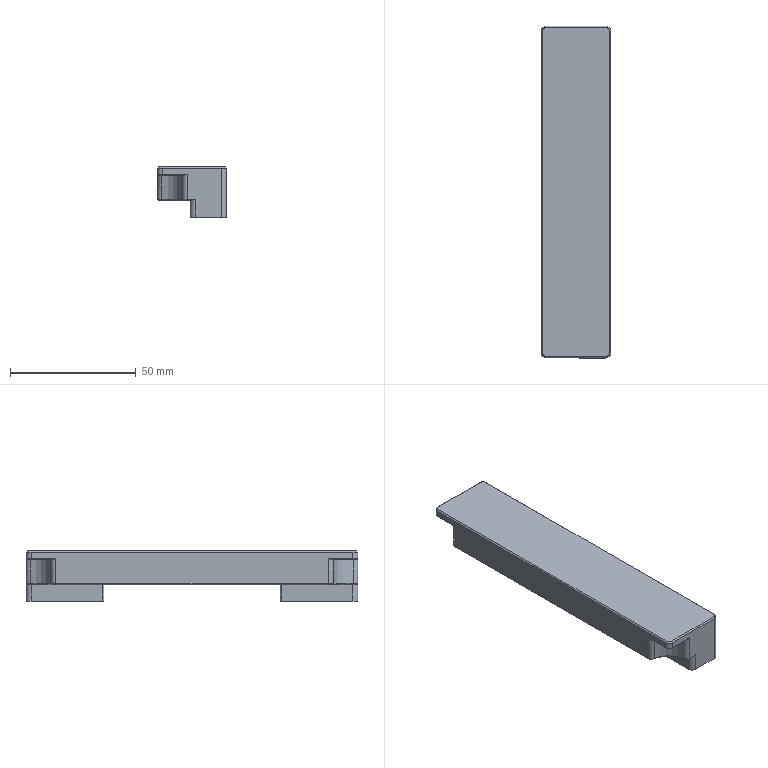NC program | NX | posted with a generic post | part box 27.5 x 132 x 20 mm
Lines 1 to 18 of 2947:
N10 G17 G21 G94 G90
(FLOOR_WALL , TOOL : D80)
N12 T19 M6
N14 G54
N16 G17 G0 G90 X-111. Y0. S6500 M3
N18 G43 Z30. H19
N20 Z3.
N22 G94 G1 Z0. F1500.
N24 X-108.
N26 X108.
N28 X111.
N30 Z3.
N32 G0 Z30.
N34 M5